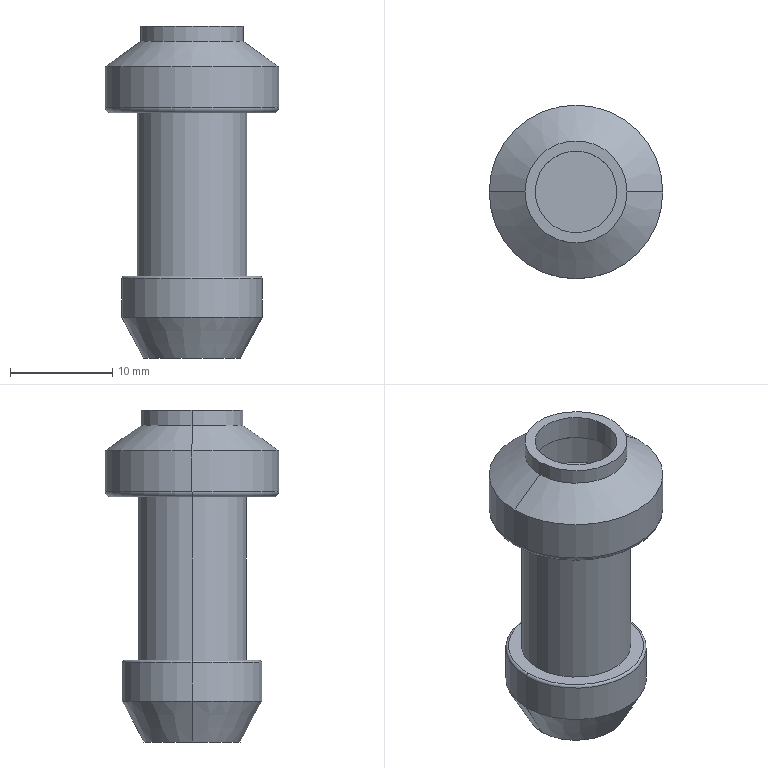Part | SolidWorks | features BaseBody 1 | 1 solid | 35 faces | box 17 x 17 x 32.5 mm | volume 1549 mm3 | cylinder 16 | cone 8 | plane 7 | torus 4 | commonest cylinder face diameters 8 x2 8.7 x2 10 x2 10.7 x2 11.75 x2 13.75 x2
STEP:
#1=CARTESIAN_POINT('',(-6.875,4.25,-8.5));
#2=VERTEX_POINT('',#1);
#3=CARTESIAN_POINT('',(-6.875,4.25,-12.25));
#4=VERTEX_POINT('',#3);
#5=CARTESIAN_POINT('',(-6.875,4.25,-8.25));
#6=DIRECTION('',(0.,0.,-1.));
#7=VECTOR('',#6,1000.);
#8=LINE('',#5,#7);
#9=EDGE_CURVE('',#2,#4,#8,.T.);
#10=ORIENTED_EDGE('',*,*,#9,.T.);
#11=CARTESIAN_POINT('',(6.875,4.25,-12.25));
#12=VERTEX_POINT('',#11);
#13=CARTESIAN_POINT('',(0.,4.25,-12.25));
#14=DIRECTION('',(0.,0.,1.));
#15=DIRECTION('',(1.,0.,0.));
#16=AXIS2_PLACEMENT_3D('',#13,#14,#15);
#17=CIRCLE('',#16,6.875);
#18=EDGE_CURVE('',#4,#12,#17,.T.);
#19=ORIENTED_EDGE('',*,*,#18,.T.);
#20=CARTESIAN_POINT('',(6.875,4.25,-8.5));
#21=VERTEX_POINT('',#20);
#22=CARTESIAN_POINT('',(6.875,4.25,-8.25));
#23=DIRECTION('',(0.,0.,-1.));
#24=VECTOR('',#23,1000.);
#25=LINE('',#22,#24);
#26=EDGE_CURVE('',#21,#12,#25,.T.);
#27=ORIENTED_EDGE('',*,*,#26,.F.);
#28=CARTESIAN_POINT('',(0.,4.25,-8.5));
#29=DIRECTION('',(0.,0.,1.));
#30=DIRECTION('',(1.,0.,0.));
#31=AXIS2_PLACEMENT_3D('',#28,#29,#30);
#32=CIRCLE('',#31,6.875);
#33=EDGE_CURVE('',#2,#21,#32,.T.);
#34=ORIENTED_EDGE('',*,*,#33,.F.);
#35=EDGE_LOOP('',(#10,#19,#27,#34));
#36=FACE_OUTER_BOUND('',#35,.T.);
#37=CARTESIAN_POINT('',(0.,4.25,-8.25));
#38=DIRECTION('',(0.,0.,-1.));
#39=DIRECTION('',(1.,0.,0.));
#40=AXIS2_PLACEMENT_3D('',#37,#38,#39);
#41=CYLINDRICAL_SURFACE('',#40,6.875);
#42=ADVANCED_FACE('',(#36),#41,.T.);
#43=CARTESIAN_POINT('',(4.75,4.25,-16.25));
#44=VERTEX_POINT('',#43);
#45=CARTESIAN_POINT('',(4.75,4.25,-16.25));
#46=DIRECTION('',(0.4692,0.,0.8831));
#47=VECTOR('',#46,1000.);
#48=LINE('',#45,#47);
#49=EDGE_CURVE('',#44,#12,#48,.T.);
#50=ORIENTED_EDGE('',*,*,#49,.T.);
#51=ORIENTED_EDGE('',*,*,#18,.F.);
#52=CARTESIAN_POINT('',(-4.75,4.25,-16.25));
#53=VERTEX_POINT('',#52);
#54=CARTESIAN_POINT('',(-4.75,4.25,-16.25));
#55=DIRECTION('',(-0.4692,0.,0.8831));
#56=VECTOR('',#55,1000.);
#57=LINE('',#54,#56);
#58=EDGE_CURVE('',#53,#4,#57,.T.);
#59=ORIENTED_EDGE('',*,*,#58,.F.);
#60=CARTESIAN_POINT('',(0.,4.25,-16.25));
#61=DIRECTION('',(0.,0.,1.));
#62=DIRECTION('',(1.,0.,0.));
#63=AXIS2_PLACEMENT_3D('',#60,#61,#62);
#64=CIRCLE('',#63,4.75);
#65=EDGE_CURVE('',#53,#44,#64,.T.);
#66=ORIENTED_EDGE('',*,*,#65,.T.);
#67=EDGE_LOOP('',(#50,#51,#59,#66));
#68=FACE_OUTER_BOUND('',#67,.T.);
#69=CARTESIAN_POINT('',(0.,4.25,-16.25));
#70=DIRECTION('',(0.,0.,1.));
#71=DIRECTION('',(-1.,0.,0.));
#72=AXIS2_PLACEMENT_3D('',#69,#70,#71);
#73=CONICAL_SURFACE('',#72,4.75,0.4883);
#74=ADVANCED_FACE('',(#68),#73,.T.);
#75=ORIENTED_EDGE('',*,*,#65,.F.);
#76=CARTESIAN_POINT('',(0.,4.25,-16.25));
#77=DIRECTION('',(0.,0.,1.));
#78=DIRECTION('',(1.,0.,0.));
#79=AXIS2_PLACEMENT_3D('',#76,#77,#78);
#80=CIRCLE('',#79,4.75);
#81=EDGE_CURVE('',#44,#53,#80,.T.);
#82=ORIENTED_EDGE('',*,*,#81,.F.);
#83=EDGE_LOOP('',(#75,#82));
#84=FACE_OUTER_BOUND('',#83,.T.);
#85=CARTESIAN_POINT('',(0.,4.25,-16.25));
#86=DIRECTION('',(0.,0.,-1.));
#87=DIRECTION('',(0.,-1.,0.));
#88=AXIS2_PLACEMENT_3D('',#85,#86,#87);
#89=PLANE('',#88);
#90=ADVANCED_FACE('',(#84),#89,.T.);
#91=CARTESIAN_POINT('',(-4.149,4.25,-15.25));
#92=VERTEX_POINT('',#91);
#93=CARTESIAN_POINT('',(4.149,4.25,-15.25));
#94=VERTEX_POINT('',#93);
#95=CARTESIAN_POINT('',(0.,4.25,-15.25));
#96=DIRECTION('',(0.,0.,1.));
#97=DIRECTION('',(1.,0.,0.));
#98=AXIS2_PLACEMENT_3D('',#95,#96,#97);
#99=CIRCLE('',#98,4.149);
#100=EDGE_CURVE('',#92,#94,#99,.T.);
#101=ORIENTED_EDGE('',*,*,#100,.T.);
#102=CARTESIAN_POINT('',(0.,4.25,-15.25));
#103=DIRECTION('',(0.,0.,1.));
#104=DIRECTION('',(1.,0.,0.));
#105=AXIS2_PLACEMENT_3D('',#102,#103,#104);
#106=CIRCLE('',#105,4.149);
#107=EDGE_CURVE('',#94,#92,#106,.T.);
#108=ORIENTED_EDGE('',*,*,#107,.T.);
#109=EDGE_LOOP('',(#101,#108));
#110=FACE_OUTER_BOUND('',#109,.T.);
#111=CARTESIAN_POINT('',(0.,4.25,-15.25));
#112=DIRECTION('',(0.,0.,1.));
#113=DIRECTION('',(1.,0.,0.));
#114=AXIS2_PLACEMENT_3D('',#111,#112,#113);
#115=PLANE('',#114);
#116=ADVANCED_FACE('',(#110),#115,.T.);
#117=CARTESIAN_POINT('',(5.875,4.25,-12.001));
#118=VERTEX_POINT('',#117);
#119=CARTESIAN_POINT('',(5.875,4.25,-12.001));
#120=DIRECTION('',(0.4692,0.,0.8831));
#121=VECTOR('',#120,1000.);
#122=LINE('',#119,#121);
#123=EDGE_CURVE('',#94,#118,#122,.T.);
#124=ORIENTED_EDGE('',*,*,#123,.T.);
#125=CARTESIAN_POINT('',(-5.875,4.25,-12.001));
#126=VERTEX_POINT('',#125);
#127=CARTESIAN_POINT('',(0.,4.25,-12.001));
#128=DIRECTION('',(0.,0.,1.));
#129=DIRECTION('',(1.,0.,0.));
#130=AXIS2_PLACEMENT_3D('',#127,#128,#129);
#131=CIRCLE('',#130,5.875);
#132=EDGE_CURVE('',#118,#126,#131,.T.);
#133=ORIENTED_EDGE('',*,*,#132,.T.);
#134=CARTESIAN_POINT('',(-5.875,4.25,-12.001));
#135=DIRECTION('',(-0.4692,0.,0.8831));
#136=VECTOR('',#135,1000.);
#137=LINE('',#134,#136);
#138=EDGE_CURVE('',#92,#126,#137,.T.);
#139=ORIENTED_EDGE('',*,*,#138,.F.);
#140=ORIENTED_EDGE('',*,*,#107,.F.);
#141=EDGE_LOOP('',(#124,#133,#139,#140));
#142=FACE_OUTER_BOUND('',#141,.T.);
#143=CARTESIAN_POINT('',(0.,4.25,-12.001));
#144=DIRECTION('',(0.,0.,1.));
#145=DIRECTION('',(-1.,0.,0.));
#146=AXIS2_PLACEMENT_3D('',#143,#144,#145);
#147=CONICAL_SURFACE('',#146,5.875,0.4883);
#148=ADVANCED_FACE('',(#142),#147,.F.);
#149=CARTESIAN_POINT('',(-5.875,4.25,-9.25));
#150=VERTEX_POINT('',#149);
#151=CARTESIAN_POINT('',(-5.875,4.25,-8.25));
#152=DIRECTION('',(0.,0.,-1.));
#153=VECTOR('',#152,1000.);
#154=LINE('',#151,#153);
#155=EDGE_CURVE('',#150,#126,#154,.T.);
#156=ORIENTED_EDGE('',*,*,#155,.T.);
#157=ORIENTED_EDGE('',*,*,#132,.F.);
#158=CARTESIAN_POINT('',(5.875,4.25,-9.25));
#159=VERTEX_POINT('',#158);
#160=CARTESIAN_POINT('',(5.875,4.25,-8.25));
#161=DIRECTION('',(0.,0.,-1.));
#162=VECTOR('',#161,1000.);
#163=LINE('',#160,#162);
#164=EDGE_CURVE('',#159,#118,#163,.T.);
#165=ORIENTED_EDGE('',*,*,#164,.F.);
#166=CARTESIAN_POINT('',(0.,4.25,-9.25));
#167=DIRECTION('',(0.,0.,1.));
#168=DIRECTION('',(1.,0.,0.));
#169=AXIS2_PLACEMENT_3D('',#166,#167,#168);
#170=CIRCLE('',#169,5.875);
#171=EDGE_CURVE('',#159,#150,#170,.T.);
#172=ORIENTED_EDGE('',*,*,#171,.T.);
#173=EDGE_LOOP('',(#156,#157,#165,#172));
#174=FACE_OUTER_BOUND('',#173,.T.);
#175=CARTESIAN_POINT('',(0.,4.25,-8.25));
#176=DIRECTION('',(0.,0.,-1.));
#177=DIRECTION('',(1.,0.,0.));
#178=AXIS2_PLACEMENT_3D('',#175,#176,#177);
#179=CYLINDRICAL_SURFACE('',#178,5.875);
#180=ADVANCED_FACE('',(#174),#179,.F.);
#181=CARTESIAN_POINT('',(4.35,4.25,-9.25));
#182=VERTEX_POINT('',#181);
#183=CARTESIAN_POINT('',(-4.35,4.25,-9.25));
#184=VERTEX_POINT('',#183);
#185=CARTESIAN_POINT('',(0.,4.25,-9.25));
#186=DIRECTION('',(0.,0.,1.));
#187=DIRECTION('',(1.,0.,0.));
#188=AXIS2_PLACEMENT_3D('',#185,#186,#187);
#189=CIRCLE('',#188,4.35);
#190=EDGE_CURVE('',#182,#184,#189,.T.);
#191=ORIENTED_EDGE('',*,*,#190,.T.);
#192=CARTESIAN_POINT('',(0.,4.25,-9.25));
#193=DIRECTION('',(0.,0.,1.));
#194=DIRECTION('',(1.,0.,0.));
#195=AXIS2_PLACEMENT_3D('',#192,#193,#194);
#196=CIRCLE('',#195,4.35);
#197=EDGE_CURVE('',#184,#182,#196,.T.);
#198=ORIENTED_EDGE('',*,*,#197,.T.);
#199=EDGE_LOOP('',(#191,#198));
#200=FACE_BOUND('',#199,.T.);
#201=ORIENTED_EDGE('',*,*,#171,.F.);
#202=CARTESIAN_POINT('',(0.,4.25,-9.25));
#203=DIRECTION('',(0.,0.,1.));
#204=DIRECTION('',(1.,0.,0.));
#205=AXIS2_PLACEMENT_3D('',#202,#203,#204);
#206=CIRCLE('',#205,5.875);
#207=EDGE_CURVE('',#150,#159,#206,.T.);
#208=ORIENTED_EDGE('',*,*,#207,.F.);
#209=EDGE_LOOP('',(#201,#208));
#210=FACE_OUTER_BOUND('',#209,.T.);
#211=CARTESIAN_POINT('',(0.,-0.1,-9.25));
#212=DIRECTION('',(0.,0.,-1.));
#213=DIRECTION('',(0.,-1.,0.));
#214=AXIS2_PLACEMENT_3D('',#211,#212,#213);
#215=PLANE('',#214);
#216=ADVANCED_FACE('',(#200,#210),#215,.T.);
#217=CARTESIAN_POINT('',(-4.35,4.25,8.75));
#218=VERTEX_POINT('',#217);
#219=CARTESIAN_POINT('',(-4.35,4.25,-8.25));
#220=DIRECTION('',(0.,0.,-1.));
#221=VECTOR('',#220,1000.);
#222=LINE('',#219,#221);
#223=EDGE_CURVE('',#218,#184,#222,.T.);
#224=ORIENTED_EDGE('',*,*,#223,.T.);
#225=ORIENTED_EDGE('',*,*,#190,.F.);
#226=CARTESIAN_POINT('',(4.35,4.25,8.75));
#227=VERTEX_POINT('',#226);
#228=CARTESIAN_POINT('',(4.35,4.25,-8.25));
#229=DIRECTION('',(0.,0.,-1.));
#230=VECTOR('',#229,1000.);
#231=LINE('',#228,#230);
#232=EDGE_CURVE('',#227,#182,#231,.T.);
#233=ORIENTED_EDGE('',*,*,#232,.F.);
#234=CARTESIAN_POINT('',(0.,4.25,8.75));
#235=DIRECTION('',(0.,0.,1.));
#236=DIRECTION('',(1.,0.,0.));
#237=AXIS2_PLACEMENT_3D('',#234,#235,#236);
#238=CIRCLE('',#237,4.35);
#239=EDGE_CURVE('',#227,#218,#238,.T.);
#240=ORIENTED_EDGE('',*,*,#239,.T.);
#241=EDGE_LOOP('',(#224,#225,#233,#240));
#242=FACE_OUTER_BOUND('',#241,.T.);
#243=CARTESIAN_POINT('',(0.,4.25,-8.25));
#244=DIRECTION('',(0.,0.,-1.));
#245=DIRECTION('',(1.,0.,0.));
#246=AXIS2_PLACEMENT_3D('',#243,#244,#245);
#247=CYLINDRICAL_SURFACE('',#246,4.35);
#248=ADVANCED_FACE('',(#242),#247,.F.);
#249=ORIENTED_EDGE('',*,*,#239,.F.);
#250=CARTESIAN_POINT('',(0.,4.25,8.75));
#251=DIRECTION('',(0.,0.,1.));
#252=DIRECTION('',(1.,0.,0.));
#253=AXIS2_PLACEMENT_3D('',#250,#251,#252);
#254=CIRCLE('',#253,4.35);
#255=EDGE_CURVE('',#218,#227,#254,.T.);
#256=ORIENTED_EDGE('',*,*,#255,.F.);
#257=EDGE_LOOP('',(#249,#256));
#258=FACE_BOUND('',#257,.T.);
#259=CARTESIAN_POINT('',(7.,4.25,8.75));
#260=VERTEX_POINT('',#259);
#261=CARTESIAN_POINT('',(-7.,4.25,8.75));
#262=VERTEX_POINT('',#261);
#263=CARTESIAN_POINT('',(0.,4.25,8.75));
#264=DIRECTION('',(0.,0.,1.));
#265=DIRECTION('',(1.,0.,0.));
#266=AXIS2_PLACEMENT_3D('',#263,#264,#265);
#267=CIRCLE('',#266,7.);
#268=EDGE_CURVE('',#260,#262,#267,.T.);
#269=ORIENTED_EDGE('',*,*,#268,.T.);
#270=CARTESIAN_POINT('',(0.,4.25,8.75));
#271=DIRECTION('',(0.,0.,1.));
#272=DIRECTION('',(1.,0.,0.));
#273=AXIS2_PLACEMENT_3D('',#270,#271,#272);
#274=CIRCLE('',#273,7.);
#275=EDGE_CURVE('',#262,#260,#274,.T.);
#276=ORIENTED_EDGE('',*,*,#275,.T.);
#277=EDGE_LOOP('',(#269,#276));
#278=FACE_OUTER_BOUND('',#277,.T.);
#279=CARTESIAN_POINT('',(0.,-0.1,8.75));
#280=DIRECTION('',(0.,0.,1.));
#281=DIRECTION('',(1.,0.,0.));
#282=AXIS2_PLACEMENT_3D('',#279,#280,#281);
#283=PLANE('',#282);
#284=ADVANCED_FACE('',(#258,#278),#283,.T.);
#285=CARTESIAN_POINT('',(-7.,4.25,11.735));
#286=VERTEX_POINT('',#285);
#287=CARTESIAN_POINT('',(-7.,4.25,-8.25));
#288=DIRECTION('',(0.,0.,-1.));
#289=VECTOR('',#288,1000.);
#290=LINE('',#287,#289);
#291=EDGE_CURVE('',#286,#262,#290,.T.);
#292=ORIENTED_EDGE('',*,*,#291,.T.);
#293=ORIENTED_EDGE('',*,*,#268,.F.);
#294=CARTESIAN_POINT('',(7.,4.25,11.735));
#295=VERTEX_POINT('',#294);
#296=CARTESIAN_POINT('',(7.,4.25,-8.25));
#297=DIRECTION('',(0.,0.,-1.));
#298=VECTOR('',#297,1000.);
#299=LINE('',#296,#298);
#300=EDGE_CURVE('',#295,#260,#299,.T.);
#301=ORIENTED_EDGE('',*,*,#300,.F.);
#302=CARTESIAN_POINT('',(0.,4.25,11.735));
#303=DIRECTION('',(0.,0.,1.));
#304=DIRECTION('',(1.,0.,0.));
#305=AXIS2_PLACEMENT_3D('',#302,#303,#304);
#306=CIRCLE('',#305,7.);
#307=EDGE_CURVE('',#295,#286,#306,.T.);
#308=ORIENTED_EDGE('',*,*,#307,.T.);
#309=EDGE_LOOP('',(#292,#293,#301,#308));
#310=FACE_OUTER_BOUND('',#309,.T.);
#311=CARTESIAN_POINT('',(0.,4.25,-8.25));
#312=DIRECTION('',(0.,0.,-1.));
#313=DIRECTION('',(1.,0.,0.));
#314=AXIS2_PLACEMENT_3D('',#311,#312,#313);
#315=CYLINDRICAL_SURFACE('',#314,7.);
#316=ADVANCED_FACE('',(#310),#315,.F.);
#317=CARTESIAN_POINT('',(-4.,4.25,13.878));
#318=VERTEX_POINT('',#317);
#319=CARTESIAN_POINT('',(-4.,4.25,13.878));
#320=DIRECTION('',(-0.8137,0.,-0.5812));
#321=VECTOR('',#320,1000.);
#322=LINE('',#319,#321);
#323=EDGE_CURVE('',#318,#286,#322,.T.);
#324=ORIENTED_EDGE('',*,*,#323,.T.);
#325=ORIENTED_EDGE('',*,*,#307,.F.);
#326=CARTESIAN_POINT('',(4.,4.25,13.878));
#327=VERTEX_POINT('',#326);
#328=CARTESIAN_POINT('',(4.,4.25,13.878));
#329=DIRECTION('',(0.8137,0.,-0.5812));
#330=VECTOR('',#329,1000.);
#331=LINE('',#328,#330);
#332=EDGE_CURVE('',#327,#295,#331,.T.);
#333=ORIENTED_EDGE('',*,*,#332,.F.);
#334=CARTESIAN_POINT('',(0.,4.25,13.878));
#335=DIRECTION('',(0.,0.,1.));
#336=DIRECTION('',(1.,0.,0.));
#337=AXIS2_PLACEMENT_3D('',#334,#335,#336);
#338=CIRCLE('',#337,4.);
#339=EDGE_CURVE('',#327,#318,#338,.T.);
#340=ORIENTED_EDGE('',*,*,#339,.T.);
#341=EDGE_LOOP('',(#324,#325,#333,#340));
#342=FACE_OUTER_BOUND('',#341,.T.);
#343=CARTESIAN_POINT('',(0.,4.25,13.878));
#344=DIRECTION('',(0.,0.,-1.));
#345=DIRECTION('',(1.,0.,0.));
#346=AXIS2_PLACEMENT_3D('',#343,#344,#345);
#347=CONICAL_SURFACE('',#346,4.,0.9505);
#348=ADVANCED_FACE('',(#342),#347,.F.);
#349=CARTESIAN_POINT('',(-4.,4.25,16.25));
#350=VERTEX_POINT('',#349);
#351=CARTESIAN_POINT('',(-4.,4.25,-8.25));
#352=DIRECTION('',(0.,0.,-1.));
#353=VECTOR('',#352,1000.);
#354=LINE('',#351,#353);
#355=EDGE_CURVE('',#350,#318,#354,.T.);
#356=ORIENTED_EDGE('',*,*,#355,.T.);
#357=ORIENTED_EDGE('',*,*,#339,.F.);
#358=CARTESIAN_POINT('',(4.,4.25,16.25));
#359=VERTEX_POINT('',#358);
#360=CARTESIAN_POINT('',(4.,4.25,-8.25));
#361=DIRECTION('',(0.,0.,-1.));
#362=VECTOR('',#361,1000.);
#363=LINE('',#360,#362);
#364=EDGE_CURVE('',#359,#327,#363,.T.);
#365=ORIENTED_EDGE('',*,*,#364,.F.);
#366=CARTESIAN_POINT('',(0.,4.25,16.25));
#367=DIRECTION('',(0.,0.,1.));
#368=DIRECTION('',(1.,0.,0.));
#369=AXIS2_PLACEMENT_3D('',#366,#367,#368);
#370=CIRCLE('',#369,4.);
#371=EDGE_CURVE('',#359,#350,#370,.T.);
#372=ORIENTED_EDGE('',*,*,#371,.T.);
#373=EDGE_LOOP('',(#356,#357,#365,#372));
#374=FACE_OUTER_BOUND('',#373,.T.);
#375=CARTESIAN_POINT('',(0.,4.25,-8.25));
#376=DIRECTION('',(0.,0.,-1.));
#377=DIRECTION('',(1.,0.,0.));
#378=AXIS2_PLACEMENT_3D('',#375,#376,#377);
#379=CYLINDRICAL_SURFACE('',#378,4.);
#380=ADVANCED_FACE('',(#374),#379,.F.);
#381=ORIENTED_EDGE('',*,*,#371,.F.);
#382=CARTESIAN_POINT('',(0.,4.25,16.25));
#383=DIRECTION('',(0.,0.,1.));
#384=DIRECTION('',(1.,0.,0.));
#385=AXIS2_PLACEMENT_3D('',#382,#383,#384);
#386=CIRCLE('',#385,4.);
#387=EDGE_CURVE('',#350,#359,#386,.T.);
#388=ORIENTED_EDGE('',*,*,#387,.F.);
#389=EDGE_LOOP('',(#381,#388));
#390=FACE_BOUND('',#389,.T.);
#391=CARTESIAN_POINT('',(5.,4.25,16.25));
#392=VERTEX_POINT('',#391);
#393=CARTESIAN_POINT('',(-5.,4.25,16.25));
#394=VERTEX_POINT('',#393);
#395=CARTESIAN_POINT('',(0.,4.25,16.25));
#396=DIRECTION('',(0.,0.,1.));
#397=DIRECTION('',(1.,0.,0.));
#398=AXIS2_PLACEMENT_3D('',#395,#396,#397);
#399=CIRCLE('',#398,5.);
#400=EDGE_CURVE('',#392,#394,#399,.T.);
#401=ORIENTED_EDGE('',*,*,#400,.T.);
#402=CARTESIAN_POINT('',(0.,4.25,16.25));
#403=DIRECTION('',(0.,0.,1.));
#404=DIRECTION('',(1.,0.,0.));
#405=AXIS2_PLACEMENT_3D('',#402,#403,#404);
#406=CIRCLE('',#405,5.);
#407=EDGE_CURVE('',#394,#392,#406,.T.);
#408=ORIENTED_EDGE('',*,*,#407,.T.);
#409=EDGE_LOOP('',(#401,#408));
#410=FACE_OUTER_BOUND('',#409,.T.);
#411=CARTESIAN_POINT('',(0.,-0.75,16.25));
#412=DIRECTION('',(0.,0.,1.));
#413=DIRECTION('',(1.,0.,0.));
#414=AXIS2_PLACEMENT_3D('',#411,#412,#413);
#415=PLANE('',#414);
#416=ADVANCED_FACE('',(#390,#410),#415,.T.);
#417=CARTESIAN_POINT('',(-5.,4.25,14.75));
#418=VERTEX_POINT('',#417);
#419=CARTESIAN_POINT('',(-5.,4.25,-8.25));
#420=DIRECTION('',(0.,0.,-1.));
#421=VECTOR('',#420,1000.);
#422=LINE('',#419,#421);
#423=EDGE_CURVE('',#394,#418,#422,.T.);
#424=ORIENTED_EDGE('',*,*,#423,.T.);
#425=CARTESIAN_POINT('',(5.,4.25,14.75));
#426=VERTEX_POINT('',#425);
#427=CARTESIAN_POINT('',(0.,4.25,14.75));
#428=DIRECTION('',(0.,0.,1.));
#429=DIRECTION('',(1.,0.,0.));
#430=AXIS2_PLACEMENT_3D('',#427,#428,#429);
#431=CIRCLE('',#430,5.);
#432=EDGE_CURVE('',#418,#426,#431,.T.);
#433=ORIENTED_EDGE('',*,*,#432,.T.);
#434=CARTESIAN_POINT('',(5.,4.25,-8.25));
#435=DIRECTION('',(0.,0.,-1.));
#436=VECTOR('',#435,1000.);
#437=LINE('',#434,#436);
#438=EDGE_CURVE('',#392,#426,#437,.T.);
#439=ORIENTED_EDGE('',*,*,#438,.F.);
#440=ORIENTED_EDGE('',*,*,#407,.F.);
#441=EDGE_LOOP('',(#424,#433,#439,#440));
#442=FACE_OUTER_BOUND('',#441,.T.);
#443=CARTESIAN_POINT('',(0.,4.25,-8.25));
#444=DIRECTION('',(0.,0.,-1.));
#445=DIRECTION('',(1.,0.,0.));
#446=AXIS2_PLACEMENT_3D('',#443,#444,#445);
#447=CYLINDRICAL_SURFACE('',#446,5.);
#448=ADVANCED_FACE('',(#442),#447,.T.);
#449=CARTESIAN_POINT('',(-8.5,4.25,12.25));
#450=VERTEX_POINT('',#449);
#451=CARTESIAN_POINT('',(-8.5,4.25,12.25));
#452=DIRECTION('',(-0.8137,0.,-0.5812));
#453=VECTOR('',#452,1000.);
#454=LINE('',#451,#453);
#455=EDGE_CURVE('',#418,#450,#454,.T.);
#456=ORIENTED_EDGE('',*,*,#455,.T.);
#457=CARTESIAN_POINT('',(8.5,4.25,12.25));
#458=VERTEX_POINT('',#457);
#459=CARTESIAN_POINT('',(0.,4.25,12.25));
#460=DIRECTION('',(0.,0.,1.));
#461=DIRECTION('',(1.,0.,0.));
#462=AXIS2_PLACEMENT_3D('',#459,#460,#461);
#463=CIRCLE('',#462,8.5);
#464=EDGE_CURVE('',#450,#458,#463,.T.);
#465=ORIENTED_EDGE('',*,*,#464,.T.);
#466=CARTESIAN_POINT('',(8.5,4.25,12.25));
#467=DIRECTION('',(0.8137,0.,-0.5812));
#468=VECTOR('',#467,1000.);
#469=LINE('',#466,#468);
#470=EDGE_CURVE('',#426,#458,#469,.T.);
#471=ORIENTED_EDGE('',*,*,#470,.F.);
#472=ORIENTED_EDGE('',*,*,#432,.F.);
#473=EDGE_LOOP('',(#456,#465,#471,#472));
#474=FACE_OUTER_BOUND('',#473,.T.);
#475=CARTESIAN_POINT('',(0.,4.25,12.25));
#476=DIRECTION('',(0.,0.,-1.));
#477=DIRECTION('',(1.,0.,0.));
#478=AXIS2_PLACEMENT_3D('',#475,#476,#477);
#479=CONICAL_SURFACE('',#478,8.5,0.9505);
#480=ADVANCED_FACE('',(#474),#479,.T.);
#481=CARTESIAN_POINT('',(-8.5,4.25,8.25));
#482=VERTEX_POINT('',#481);
#483=CARTESIAN_POINT('',(-8.5,4.25,-8.25));
#484=DIRECTION('',(0.,0.,-1.));
#485=VECTOR('',#484,1000.);
#486=LINE('',#483,#485);
#487=EDGE_CURVE('',#450,#482,#486,.T.);
#488=ORIENTED_EDGE('',*,*,#487,.T.);
#489=CARTESIAN_POINT('',(8.5,4.25,8.25));
#490=VERTEX_POINT('',#489);
#491=CARTESIAN_POINT('',(0.,4.25,8.25));
#492=DIRECTION('',(0.,0.,1.));
#493=DIRECTION('',(1.,0.,0.));
#494=AXIS2_PLACEMENT_3D('',#491,#492,#493);
#495=CIRCLE('',#494,8.5);
#496=EDGE_CURVE('',#482,#490,#495,.T.);
#497=ORIENTED_EDGE('',*,*,#496,.T.);
#498=CARTESIAN_POINT('',(8.5,4.25,-8.25));
#499=DIRECTION('',(0.,0.,-1.));
#500=VECTOR('',#499,1000.);
#501=LINE('',#498,#500);
#502=EDGE_CURVE('',#458,#490,#501,.T.);
#503=ORIENTED_EDGE('',*,*,#502,.F.);
#504=ORIENTED_EDGE('',*,*,#464,.F.);
#505=EDGE_LOOP('',(#488,#497,#503,#504));
#506=FACE_OUTER_BOUND('',#505,.T.);
#507=CARTESIAN_POINT('',(0.,4.25,-8.25));
#508=DIRECTION('',(0.,0.,-1.));
#509=DIRECTION('',(1.,0.,0.));
#510=AXIS2_PLACEMENT_3D('',#507,#508,#509);
#511=CYLINDRICAL_SURFACE('',#510,8.5);
#512=ADVANCED_FACE('',(#506),#511,.T.);
#513=CARTESIAN_POINT('',(-8.,4.25,7.75));
#514=VERTEX_POINT('',#513);
#515=CARTESIAN_POINT('',(-8.,4.25,8.25));
#516=DIRECTION('',(0.,-1.,0.));
#517=DIRECTION('',(-1.,0.,0.));
#518=AXIS2_PLACEMENT_3D('',#515,#516,#517);
#519=CIRCLE('',#518,0.5);
#520=EDGE_CURVE('',#482,#514,#519,.T.);
#521=ORIENTED_EDGE('',*,*,#520,.T.);
#522=CARTESIAN_POINT('',(8.,4.25,7.75));
#523=VERTEX_POINT('',#522);
#524=CARTESIAN_POINT('',(0.,4.25,7.75));
#525=DIRECTION('',(0.,0.,1.));
#526=DIRECTION('',(1.,0.,0.));
#527=AXIS2_PLACEMENT_3D('',#524,#525,#526);
#528=CIRCLE('',#527,8.);
#529=EDGE_CURVE('',#514,#523,#528,.T.);
#530=ORIENTED_EDGE('',*,*,#529,.T.);
#531=CARTESIAN_POINT('',(8.,4.25,8.25));
#532=DIRECTION('',(0.,1.,0.));
#533=DIRECTION('',(0.,0.,1.));
#534=AXIS2_PLACEMENT_3D('',#531,#532,#533);
#535=CIRCLE('',#534,0.5);
#536=EDGE_CURVE('',#490,#523,#535,.T.);
#537=ORIENTED_EDGE('',*,*,#536,.F.);
#538=ORIENTED_EDGE('',*,*,#496,.F.);
#539=EDGE_LOOP('',(#521,#530,#537,#538));
#540=FACE_OUTER_BOUND('',#539,.T.);
#541=CARTESIAN_POINT('',(0.,4.25,8.25));
#542=DIRECTION('',(0.,0.,-1.));
#543=DIRECTION('',(1.,0.,0.));
#544=AXIS2_PLACEMENT_3D('',#541,#542,#543);
#545=TOROIDAL_SURFACE('',#544,8.,0.5);
#546=ADVANCED_FACE('',(#540),#545,.T.);
#547=CARTESIAN_POINT('',(5.35,4.25,7.75));
#548=VERTEX_POINT('',#547);
#549=CARTESIAN_POINT('',(-5.35,4.25,7.75));
#550=VERTEX_POINT('',#549);
#551=CARTESIAN_POINT('',(0.,4.25,7.75));
#552=DIRECTION('',(0.,0.,1.));
#553=DIRECTION('',(1.,0.,0.));
#554=AXIS2_PLACEMENT_3D('',#551,#552,#553);
#555=CIRCLE('',#554,5.35);
#556=EDGE_CURVE('',#548,#550,#555,.T.);
#557=ORIENTED_EDGE('',*,*,#556,.T.);
#558=CARTESIAN_POINT('',(0.,4.25,7.75));
#559=DIRECTION('',(0.,0.,1.));
#560=DIRECTION('',(1.,0.,0.));
#561=AXIS2_PLACEMENT_3D('',#558,#559,#560);
#562=CIRCLE('',#561,5.35);
#563=EDGE_CURVE('',#550,#548,#562,.T.);
#564=ORIENTED_EDGE('',*,*,#563,.T.);
#565=EDGE_LOOP('',(#557,#564));
#566=FACE_BOUND('',#565,.T.);
#567=CARTESIAN_POINT('',(0.,4.25,7.75));
#568=DIRECTION('',(0.,0.,1.));
#569=DIRECTION('',(1.,0.,0.));
#570=AXIS2_PLACEMENT_3D('',#567,#568,#569);
#571=CIRCLE('',#570,8.);
#572=EDGE_CURVE('',#523,#514,#571,.T.);
#573=ORIENTED_EDGE('',*,*,#572,.F.);
#574=ORIENTED_EDGE('',*,*,#529,.F.);
#575=EDGE_LOOP('',(#573,#574));
#576=FACE_OUTER_BOUND('',#575,.T.);
#577=CARTESIAN_POINT('',(0.,-1.1,7.75));
#578=DIRECTION('',(0.,0.,-1.));
#579=DIRECTION('',(0.,-1.,0.));
#580=AXIS2_PLACEMENT_3D('',#577,#578,#579);
#581=PLANE('',#580);
#582=ADVANCED_FACE('',(#566,#576),#581,.T.);
#583=CARTESIAN_POINT('',(-5.35,4.25,-8.25));
#584=VERTEX_POINT('',#583);
#585=CARTESIAN_POINT('',(-5.35,4.25,-8.25));
#586=DIRECTION('',(0.,0.,-1.));
#587=VECTOR('',#586,1000.);
#588=LINE('',#585,#587);
#589=EDGE_CURVE('',#550,#584,#588,.T.);
#590=ORIENTED_EDGE('',*,*,#589,.T.);
#591=CARTESIAN_POINT('',(5.35,4.25,-8.25));
#592=VERTEX_POINT('',#591);
#593=CARTESIAN_POINT('',(0.,4.25,-8.25));
#594=DIRECTION('',(0.,0.,1.));
#595=DIRECTION('',(1.,0.,0.));
#596=AXIS2_PLACEMENT_3D('',#593,#594,#595);
#597=CIRCLE('',#596,5.35);
#598=EDGE_CURVE('',#584,#592,#597,.T.);
#599=ORIENTED_EDGE('',*,*,#598,.T.);
#600=CARTESIAN_POINT('',(5.35,4.25,-8.25));
#601=DIRECTION('',(0.,0.,-1.));
#602=VECTOR('',#601,1000.);
#603=LINE('',#600,#602);
#604=EDGE_CURVE('',#548,#592,#603,.T.);
#605=ORIENTED_EDGE('',*,*,#604,.F.);
#606=ORIENTED_EDGE('',*,*,#563,.F.);
#607=EDGE_LOOP('',(#590,#599,#605,#606));
#608=FACE_OUTER_BOUND('',#607,.T.);
#609=CARTESIAN_POINT('',(0.,4.25,-8.25));
#610=DIRECTION('',(0.,0.,-1.));
#611=DIRECTION('',(1.,0.,0.));
#612=AXIS2_PLACEMENT_3D('',#609,#610,#611);
#613=CYLINDRICAL_SURFACE('',#612,5.35);
#614=ADVANCED_FACE('',(#608),#613,.T.);
#615=CARTESIAN_POINT('',(0.,4.25,-8.25));
#616=DIRECTION('',(0.,0.,1.));
#617=DIRECTION('',(1.,0.,0.));
#618=AXIS2_PLACEMENT_3D('',#615,#616,#617);
#619=CIRCLE('',#618,5.35);
#620=EDGE_CURVE('',#592,#584,#619,.T.);
#621=ORIENTED_EDGE('',*,*,#620,.F.);
#622=ORIENTED_EDGE('',*,*,#598,.F.);
#623=EDGE_LOOP('',(#621,#622));
#624=FACE_BOUND('',#623,.T.);
#625=CARTESIAN_POINT('',(6.625,4.25,-8.25));
#626=VERTEX_POINT('',#625);
#627=CARTESIAN_POINT('',(-6.625,4.25,-8.25));
#628=VERTEX_POINT('',#627);
#629=CARTESIAN_POINT('',(0.,4.25,-8.25));
#630=DIRECTION('',(0.,0.,1.));
#631=DIRECTION('',(1.,0.,0.));
#632=AXIS2_PLACEMENT_3D('',#629,#630,#631);
#633=CIRCLE('',#632,6.625);
#634=EDGE_CURVE('',#626,#628,#633,.T.);
#635=ORIENTED_EDGE('',*,*,#634,.T.);
#636=CARTESIAN_POINT('',(0.,4.25,-8.25));
#637=DIRECTION('',(0.,0.,1.));
#638=DIRECTION('',(1.,0.,0.));
#639=AXIS2_PLACEMENT_3D('',#636,#637,#638);
#640=CIRCLE('',#639,6.625);
#641=EDGE_CURVE('',#628,#626,#640,.T.);
#642=ORIENTED_EDGE('',*,*,#641,.T.);
#643=EDGE_LOOP('',(#635,#642));
#644=FACE_OUTER_BOUND('',#643,.T.);
#645=CARTESIAN_POINT('',(0.,-1.1,-8.25));
#646=DIRECTION('',(0.,0.,1.));
#647=DIRECTION('',(1.,0.,0.));
#648=AXIS2_PLACEMENT_3D('',#645,#646,#647);
#649=PLANE('',#648);
#650=ADVANCED_FACE('',(#624,#644),#649,.T.);
#651=CARTESIAN_POINT('',(-6.625,4.25,-8.5));
#652=DIRECTION('',(0.,-1.,0.));
#653=DIRECTION('',(-1.,0.,0.));
#654=AXIS2_PLACEMENT_3D('',#651,#652,#653);
#655=CIRCLE('',#654,0.25);
#656=EDGE_CURVE('',#628,#2,#655,.T.);
#657=ORIENTED_EDGE('',*,*,#656,.T.);
#658=ORIENTED_EDGE('',*,*,#33,.T.);
#659=CARTESIAN_POINT('',(6.625,4.25,-8.5));
#660=DIRECTION('',(0.,1.,0.));
#661=DIRECTION('',(0.,0.,1.));
#662=AXIS2_PLACEMENT_3D('',#659,#660,#661);
#663=CIRCLE('',#662,0.25);
#664=EDGE_CURVE('',#626,#21,#663,.T.);
#665=ORIENTED_EDGE('',*,*,#664,.F.);
#666=ORIENTED_EDGE('',*,*,#641,.F.);
#667=EDGE_LOOP('',(#657,#658,#665,#666));
#668=FACE_OUTER_BOUND('',#667,.T.);
#669=CARTESIAN_POINT('',(0.,4.25,-8.5));
#670=DIRECTION('',(0.,0.,-1.));
#671=DIRECTION('',(1.,0.,0.));
#672=AXIS2_PLACEMENT_3D('',#669,#670,#671);
#673=TOROIDAL_SURFACE('',#672,6.625,0.25);
#674=ADVANCED_FACE('',(#668),#673,.T.);
#675=ORIENTED_EDGE('',*,*,#634,.F.);
#676=ORIENTED_EDGE('',*,*,#664,.T.);
#677=CARTESIAN_POINT('',(0.,4.25,-8.5));
#678=DIRECTION('',(0.,0.,1.));
#679=DIRECTION('',(1.,0.,0.));
#680=AXIS2_PLACEMENT_3D('',#677,#678,#679);
#681=CIRCLE('',#680,6.875);
#682=EDGE_CURVE('',#21,#2,#681,.T.);
#683=ORIENTED_EDGE('',*,*,#682,.T.);
#684=ORIENTED_EDGE('',*,*,#656,.F.);
#685=EDGE_LOOP('',(#675,#676,#683,#684));
#686=FACE_OUTER_BOUND('',#685,.T.);
#687=CARTESIAN_POINT('',(0.,4.25,-8.5));
#688=DIRECTION('',(0.,0.,-1.));
#689=DIRECTION('',(1.,0.,0.));
#690=AXIS2_PLACEMENT_3D('',#687,#688,#689);
#691=TOROIDAL_SURFACE('',#690,6.625,0.25);
#692=ADVANCED_FACE('',(#686),#691,.T.);
#693=ORIENTED_EDGE('',*,*,#556,.F.);
#694=ORIENTED_EDGE('',*,*,#604,.T.);
#695=ORIENTED_EDGE('',*,*,#620,.T.);
#696=ORIENTED_EDGE('',*,*,#589,.F.);
#697=EDGE_LOOP('',(#693,#694,#695,#696));
#698=FACE_OUTER_BOUND('',#697,.T.);
#699=CARTESIAN_POINT('',(0.,4.25,-8.25));
#700=DIRECTION('',(0.,0.,-1.));
#701=DIRECTION('',(1.,0.,0.));
#702=AXIS2_PLACEMENT_3D('',#699,#700,#701);
#703=CYLINDRICAL_SURFACE('',#702,5.35);
#704=ADVANCED_FACE('',(#698),#703,.T.);
#705=CARTESIAN_POINT('',(0.,4.25,8.25));
#706=DIRECTION('',(0.,0.,1.));
#707=DIRECTION('',(1.,0.,0.));
#708=AXIS2_PLACEMENT_3D('',#705,#706,#707);
#709=CIRCLE('',#708,8.5);
#710=EDGE_CURVE('',#490,#482,#709,.T.);
#711=ORIENTED_EDGE('',*,*,#710,.F.);
#712=ORIENTED_EDGE('',*,*,#536,.T.);
#713=ORIENTED_EDGE('',*,*,#572,.T.);
#714=ORIENTED_EDGE('',*,*,#520,.F.);
#715=EDGE_LOOP('',(#711,#712,#713,#714));
#716=FACE_OUTER_BOUND('',#715,.T.);
#717=CARTESIAN_POINT('',(0.,4.25,8.25));
#718=DIRECTION('',(0.,0.,-1.));
#719=DIRECTION('',(1.,0.,0.));
#720=AXIS2_PLACEMENT_3D('',#717,#718,#719);
#721=TOROIDAL_SURFACE('',#720,8.,0.5);
#722=ADVANCED_FACE('',(#716),#721,.T.);
#723=CARTESIAN_POINT('',(0.,4.25,12.25));
#724=DIRECTION('',(0.,0.,1.));
#725=DIRECTION('',(1.,0.,0.));
#726=AXIS2_PLACEMENT_3D('',#723,#724,#725);
#727=CIRCLE('',#726,8.5);
#728=EDGE_CURVE('',#458,#450,#727,.T.);
#729=ORIENTED_EDGE('',*,*,#728,.F.);
#730=ORIENTED_EDGE('',*,*,#502,.T.);
#731=ORIENTED_EDGE('',*,*,#710,.T.);
#732=ORIENTED_EDGE('',*,*,#487,.F.);
#733=EDGE_LOOP('',(#729,#730,#731,#732));
#734=FACE_OUTER_BOUND('',#733,.T.);
#735=CARTESIAN_POINT('',(0.,4.25,-8.25));
#736=DIRECTION('',(0.,0.,-1.));
#737=DIRECTION('',(1.,0.,0.));
#738=AXIS2_PLACEMENT_3D('',#735,#736,#737);
#739=CYLINDRICAL_SURFACE('',#738,8.5);
#740=ADVANCED_FACE('',(#734),#739,.T.);
#741=CARTESIAN_POINT('',(0.,4.25,14.75));
#742=DIRECTION('',(0.,0.,1.));
#743=DIRECTION('',(1.,0.,0.));
#744=AXIS2_PLACEMENT_3D('',#741,#742,#743);
#745=CIRCLE('',#744,5.);
#746=EDGE_CURVE('',#426,#418,#745,.T.);
#747=ORIENTED_EDGE('',*,*,#746,.F.);
#748=ORIENTED_EDGE('',*,*,#470,.T.);
#749=ORIENTED_EDGE('',*,*,#728,.T.);
#750=ORIENTED_EDGE('',*,*,#455,.F.);
#751=EDGE_LOOP('',(#747,#748,#749,#750));
#752=FACE_OUTER_BOUND('',#751,.T.);
#753=CARTESIAN_POINT('',(0.,4.25,12.25));
#754=DIRECTION('',(0.,0.,-1.));
#755=DIRECTION('',(1.,0.,0.));
#756=AXIS2_PLACEMENT_3D('',#753,#754,#755);
#757=CONICAL_SURFACE('',#756,8.5,0.9505);
#758=ADVANCED_FACE('',(#752),#757,.T.);
#759=ORIENTED_EDGE('',*,*,#400,.F.);
#760=ORIENTED_EDGE('',*,*,#438,.T.);
#761=ORIENTED_EDGE('',*,*,#746,.T.);
#762=ORIENTED_EDGE('',*,*,#423,.F.);
#763=EDGE_LOOP('',(#759,#760,#761,#762));
#764=FACE_OUTER_BOUND('',#763,.T.);
#765=CARTESIAN_POINT('',(0.,4.25,-8.25));
#766=DIRECTION('',(0.,0.,-1.));
#767=DIRECTION('',(1.,0.,0.));
#768=AXIS2_PLACEMENT_3D('',#765,#766,#767);
#769=CYLINDRICAL_SURFACE('',#768,5.);
#770=ADVANCED_FACE('',(#764),#769,.T.);
#771=ORIENTED_EDGE('',*,*,#387,.T.);
#772=ORIENTED_EDGE('',*,*,#364,.T.);
#773=CARTESIAN_POINT('',(0.,4.25,13.878));
#774=DIRECTION('',(0.,0.,1.));
#775=DIRECTION('',(1.,0.,0.));
#776=AXIS2_PLACEMENT_3D('',#773,#774,#775);
#777=CIRCLE('',#776,4.);
#778=EDGE_CURVE('',#318,#327,#777,.T.);
#779=ORIENTED_EDGE('',*,*,#778,.F.);
#780=ORIENTED_EDGE('',*,*,#355,.F.);
#781=EDGE_LOOP('',(#771,#772,#779,#780));
#782=FACE_OUTER_BOUND('',#781,.T.);
#783=CARTESIAN_POINT('',(0.,4.25,-8.25));
#784=DIRECTION('',(0.,0.,-1.));
#785=DIRECTION('',(1.,0.,0.));
#786=AXIS2_PLACEMENT_3D('',#783,#784,#785);
#787=CYLINDRICAL_SURFACE('',#786,4.);
#788=ADVANCED_FACE('',(#782),#787,.F.);
#789=ORIENTED_EDGE('',*,*,#778,.T.);
#790=ORIENTED_EDGE('',*,*,#332,.T.);
#791=CARTESIAN_POINT('',(0.,4.25,11.735));
#792=DIRECTION('',(0.,0.,1.));
#793=DIRECTION('',(1.,0.,0.));
#794=AXIS2_PLACEMENT_3D('',#791,#792,#793);
#795=CIRCLE('',#794,7.);
#796=EDGE_CURVE('',#286,#295,#795,.T.);
#797=ORIENTED_EDGE('',*,*,#796,.F.);
#798=ORIENTED_EDGE('',*,*,#323,.F.);
#799=EDGE_LOOP('',(#789,#790,#797,#798));
#800=FACE_OUTER_BOUND('',#799,.T.);
#801=CARTESIAN_POINT('',(0.,4.25,13.878));
#802=DIRECTION('',(0.,0.,-1.));
#803=DIRECTION('',(1.,0.,0.));
#804=AXIS2_PLACEMENT_3D('',#801,#802,#803);
#805=CONICAL_SURFACE('',#804,4.,0.9505);
#806=ADVANCED_FACE('',(#800),#805,.F.);
#807=ORIENTED_EDGE('',*,*,#796,.T.);
#808=ORIENTED_EDGE('',*,*,#300,.T.);
#809=ORIENTED_EDGE('',*,*,#275,.F.);
#810=ORIENTED_EDGE('',*,*,#291,.F.);
#811=EDGE_LOOP('',(#807,#808,#809,#810));
#812=FACE_OUTER_BOUND('',#811,.T.);
#813=CARTESIAN_POINT('',(0.,4.25,-8.25));
#814=DIRECTION('',(0.,0.,-1.));
#815=DIRECTION('',(1.,0.,0.));
#816=AXIS2_PLACEMENT_3D('',#813,#814,#815);
#817=CYLINDRICAL_SURFACE('',#816,7.);
#818=ADVANCED_FACE('',(#812),#817,.F.);
#819=ORIENTED_EDGE('',*,*,#255,.T.);
#820=ORIENTED_EDGE('',*,*,#232,.T.);
#821=ORIENTED_EDGE('',*,*,#197,.F.);
#822=ORIENTED_EDGE('',*,*,#223,.F.);
#823=EDGE_LOOP('',(#819,#820,#821,#822));
#824=FACE_OUTER_BOUND('',#823,.T.);
#825=CARTESIAN_POINT('',(0.,4.25,-8.25));
#826=DIRECTION('',(0.,0.,-1.));
#827=DIRECTION('',(1.,0.,0.));
#828=AXIS2_PLACEMENT_3D('',#825,#826,#827);
#829=CYLINDRICAL_SURFACE('',#828,4.35);
#830=ADVANCED_FACE('',(#824),#829,.F.);
#831=ORIENTED_EDGE('',*,*,#207,.T.);
#832=ORIENTED_EDGE('',*,*,#164,.T.);
#833=CARTESIAN_POINT('',(0.,4.25,-12.001));
#834=DIRECTION('',(0.,0.,1.));
#835=DIRECTION('',(1.,0.,0.));
#836=AXIS2_PLACEMENT_3D('',#833,#834,#835);
#837=CIRCLE('',#836,5.875);
#838=EDGE_CURVE('',#126,#118,#837,.T.);
#839=ORIENTED_EDGE('',*,*,#838,.F.);
#840=ORIENTED_EDGE('',*,*,#155,.F.);
#841=EDGE_LOOP('',(#831,#832,#839,#840));
#842=FACE_OUTER_BOUND('',#841,.T.);
#843=CARTESIAN_POINT('',(0.,4.25,-8.25));
#844=DIRECTION('',(0.,0.,-1.));
#845=DIRECTION('',(1.,0.,0.));
#846=AXIS2_PLACEMENT_3D('',#843,#844,#845);
#847=CYLINDRICAL_SURFACE('',#846,5.875);
#848=ADVANCED_FACE('',(#842),#847,.F.);
#849=ORIENTED_EDGE('',*,*,#100,.F.);
#850=ORIENTED_EDGE('',*,*,#138,.T.);
#851=ORIENTED_EDGE('',*,*,#838,.T.);
#852=ORIENTED_EDGE('',*,*,#123,.F.);
#853=EDGE_LOOP('',(#849,#850,#851,#852));
#854=FACE_OUTER_BOUND('',#853,.T.);
#855=CARTESIAN_POINT('',(0.,4.25,-12.001));
#856=DIRECTION('',(0.,0.,1.));
#857=DIRECTION('',(-1.,0.,0.));
#858=AXIS2_PLACEMENT_3D('',#855,#856,#857);
#859=CONICAL_SURFACE('',#858,5.875,0.4883);
#860=ADVANCED_FACE('',(#854),#859,.F.);
#861=ORIENTED_EDGE('',*,*,#81,.T.);
#862=ORIENTED_EDGE('',*,*,#58,.T.);
#863=CARTESIAN_POINT('',(0.,4.25,-12.25));
#864=DIRECTION('',(0.,0.,1.));
#865=DIRECTION('',(1.,0.,0.));
#866=AXIS2_PLACEMENT_3D('',#863,#864,#865);
#867=CIRCLE('',#866,6.875);
#868=EDGE_CURVE('',#12,#4,#867,.T.);
#869=ORIENTED_EDGE('',*,*,#868,.F.);
#870=ORIENTED_EDGE('',*,*,#49,.F.);
#871=EDGE_LOOP('',(#861,#862,#869,#870));
#872=FACE_OUTER_BOUND('',#871,.T.);
#873=CARTESIAN_POINT('',(0.,4.25,-16.25));
#874=DIRECTION('',(0.,0.,1.));
#875=DIRECTION('',(-1.,0.,0.));
#876=AXIS2_PLACEMENT_3D('',#873,#874,#875);
#877=CONICAL_SURFACE('',#876,4.75,0.4883);
#878=ADVANCED_FACE('',(#872),#877,.T.);
#879=ORIENTED_EDGE('',*,*,#682,.F.);
#880=ORIENTED_EDGE('',*,*,#26,.T.);
#881=ORIENTED_EDGE('',*,*,#868,.T.);
#882=ORIENTED_EDGE('',*,*,#9,.F.);
#883=EDGE_LOOP('',(#879,#880,#881,#882));
#884=FACE_OUTER_BOUND('',#883,.T.);
#885=CARTESIAN_POINT('',(0.,4.25,-8.25));
#886=DIRECTION('',(0.,0.,-1.));
#887=DIRECTION('',(1.,0.,0.));
#888=AXIS2_PLACEMENT_3D('',#885,#886,#887);
#889=CYLINDRICAL_SURFACE('',#888,6.875);
#890=ADVANCED_FACE('',(#884),#889,.T.);
#891=CLOSED_SHELL('',(#42,#74,#90,#116,#148,#180,#216,#248,#284,#316,#348,#380,#416,#448,#480,#512,#546,#582,#614,#650,#674,#692,#704,#722,#740,#758,#770,#788,#806,#818,#830,#848,#860,#878,#890));
#892=MANIFOLD_SOLID_BREP('',#891);
#893=CARTESIAN_POINT('',(0.,0.,0.));
#894=DIRECTION('',(0.,0.,1.));
#895=DIRECTION('',(1.,0.,0.));
#896=AXIS2_PLACEMENT_3D('',#893,#894,#895);
#897=(LENGTH_UNIT()NAMED_UNIT(*)SI_UNIT(.MILLI.,.METRE.));
#898=UNCERTAINTY_MEASURE_WITH_UNIT(LENGTH_MEASURE(0.00001),#897,'','');
#899=(NAMED_UNIT(*)PLANE_ANGLE_UNIT()SI_UNIT($,.RADIAN.));
#900=(NAMED_UNIT(*)SI_UNIT($,.STERADIAN.)SOLID_ANGLE_UNIT());
#901=(GEOMETRIC_REPRESENTATION_CONTEXT(3)GLOBAL_UNCERTAINTY_ASSIGNED_CONTEXT((#898))GLOBAL_UNIT_ASSIGNED_CONTEXT((#897,#899,#900))REPRESENTATION_CONTEXT('',''));
#902=ADVANCED_BREP_SHAPE_REPRESENTATION('',(#892,#896),#901);